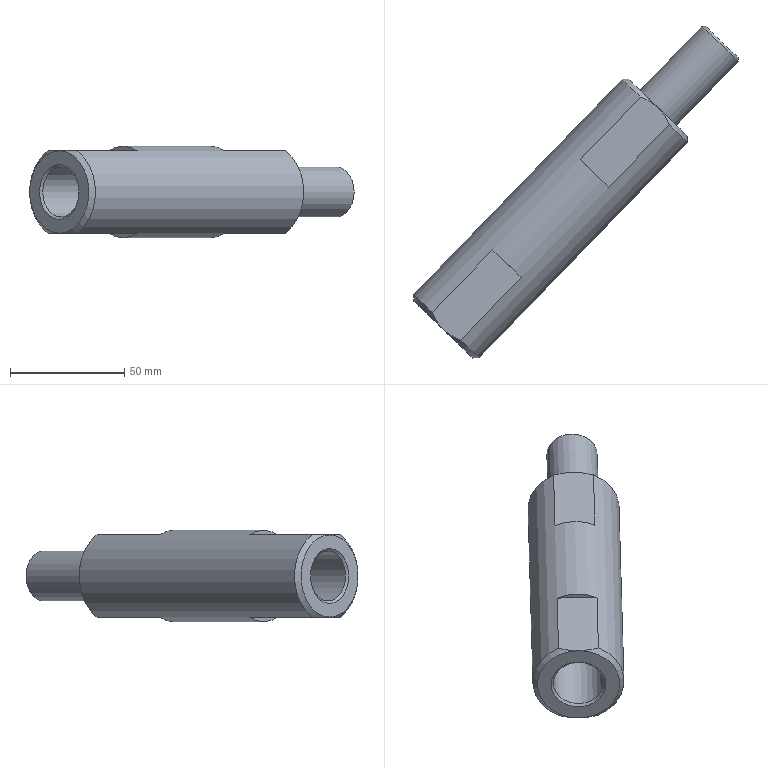Part | STEP file | HL4GZ-1.313.206 (steering cylinder extension rod) | 1 solid | 21 faces | box 141.883 x 145.233 x 40 mm | volume 166510 mm3 | plane 11 | cone 7 | cylinder 3 | commonest cylinder face diameters 22 x2 40 x1